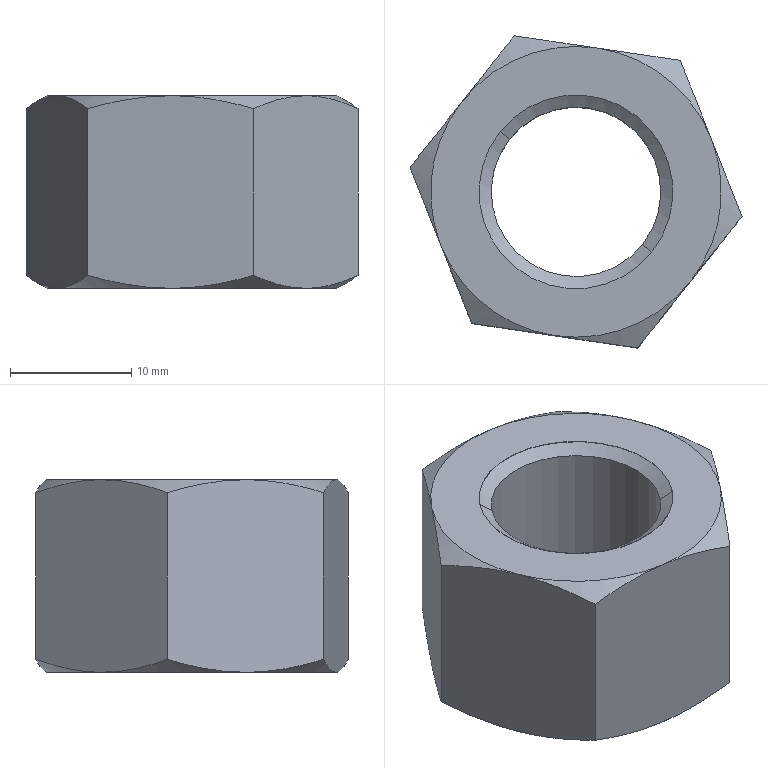Part | STEP file | Input 138 | 1 solid | 28 faces | box 27.415 x 25.769 x 15.9 mm | volume 5420 mm3 | cone 16 | plane 8 | cylinder 4 | commonest cylinder face diameters 14 x2 16 x2